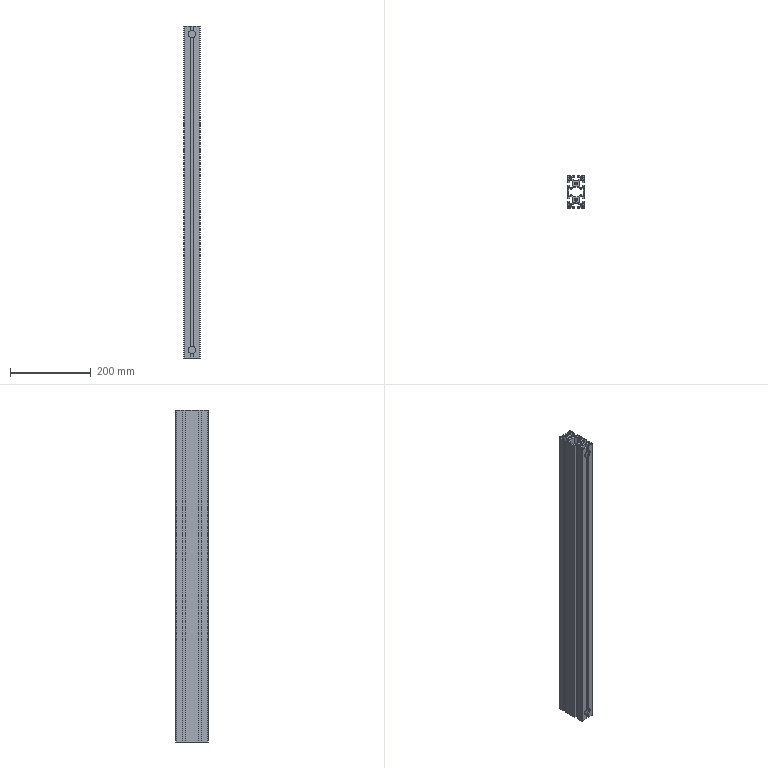Part | STEP file | 09-15 aluminium profile 4080-820 | 1 solid | 170 faces | box 40 x 80 x 820 mm | volume 984029 mm3 | plane 134 | cylinder 36 | commonest cylinder face diameters 18.5 x20 5 x8 4 x4 6.7 x4